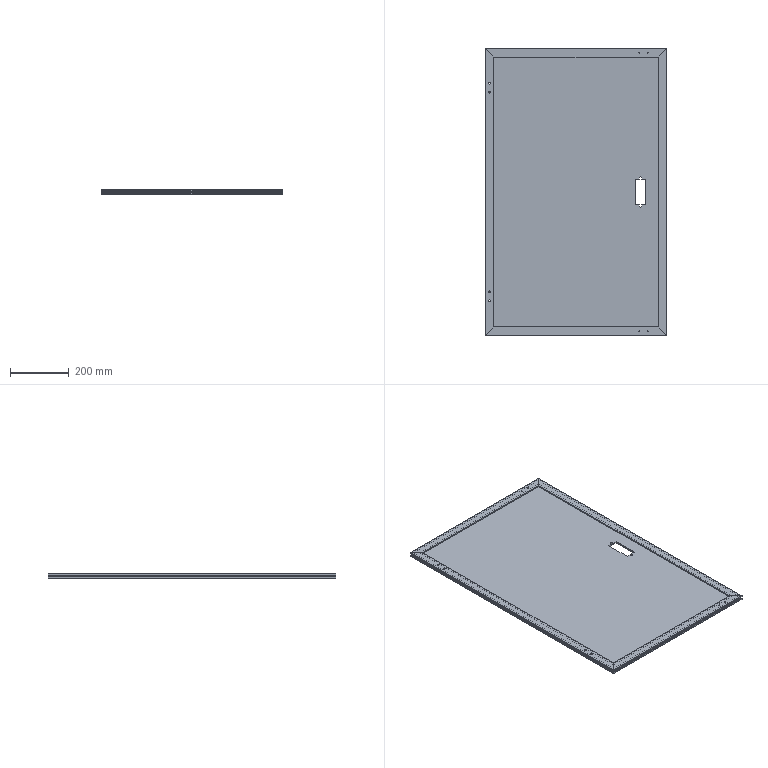Part | SolidWorks | features WeldCornerFeat 4, HoleWzd 2, ICE 2, 3DProfileFeature 1, WeldMemberFeat 1, WeldmentFeature 1 | 5 solids | 194 faces | box 618.5 x 978 x 15 mm | volume 4035765 mm3 | plane 136 | cylinder 50 | cone 8 | commonest cylinder face diameters 5 x32 3.3 x16 7 x2